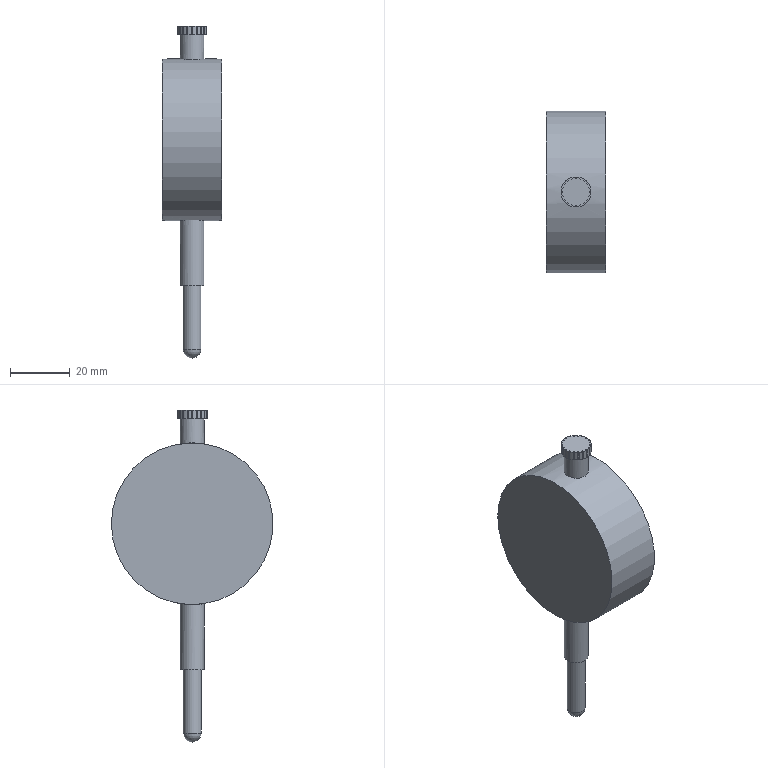Part | NX | features EXTRUDE 30, EXTRACT_STRING 24, Instance Feature 23, DATUM_CSYS 7, SKETCH 6, CYLINDER 3, DATUM_PLANE 1, OFFSET_CURVE 1, Pattern Feature 1, SPHERE 1 | 1 solid | 218 faces | box 20 x 54 x 110.9 mm | volume 44306 mm3 | plane 191 | cylinder 26 | sphere 1 | commonest cylinder face diameters 10 x20 8 x2 4 x1 6 x1 50 x1 54 x1